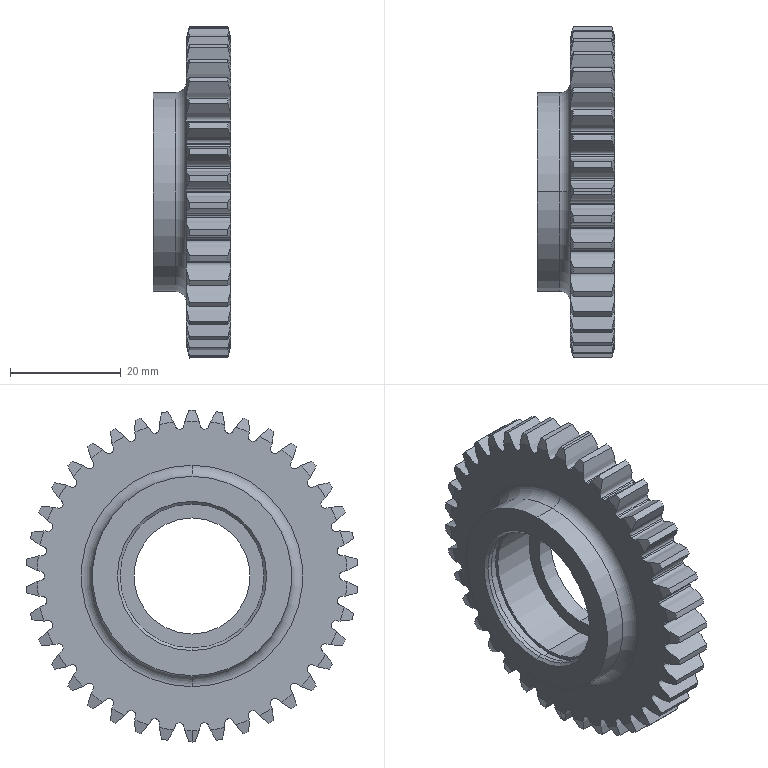Part | SolidWorks | features Chamfer 3, ICE 2, CirPattern 1, Extrusion 1, Fillet 1, RefAxis 1, RevCut 1 | 1 solid | 251 faces | box 14 x 59.878 x 60 mm | volume 19418 mm3 | cylinder 87 | cone 80 | spline 76 | plane 6 | torus 2 | commonest cylinder face diameters 60 x39 53.25 x38 26 x4 21 x2 27.2 x2 36 x2